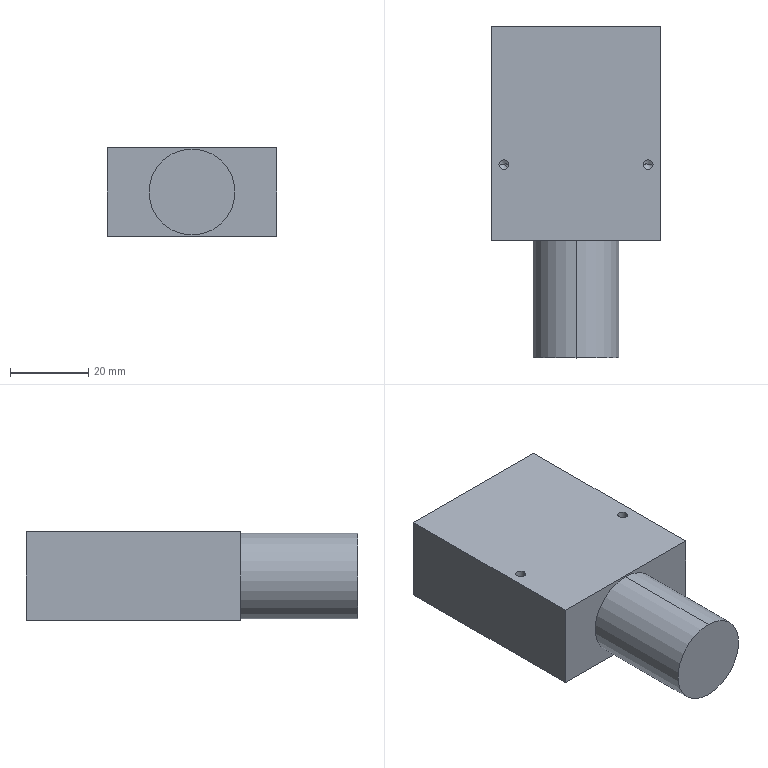Part | STEP file | Guide wheel mechanism revised.sldasm-Part-48 | 1 solid | 17 faces | box 43.5 x 85 x 22.7 mm | volume 65638 mm3 | plane 7 | cylinder 6 | cone 4 | commonest cylinder face diameters 2.5 x4 22 x2
STEP:
#1=CARTESIAN_POINT('',(0.,-30.,-11.));
#2=VERTEX_POINT('',#1);
#3=CARTESIAN_POINT('',(0.,-30.,11.));
#4=VERTEX_POINT('',#3);
#5=CARTESIAN_POINT('',(0.,-30.,0.));
#6=DIRECTION('',(0.,-1.,0.));
#7=DIRECTION('',(0.,0.,-1.));
#8=AXIS2_PLACEMENT_3D('',#5,#6,#7);
#9=CIRCLE('',#8,11.);
#10=EDGE_CURVE('',#2,#4,#9,.T.);
#11=ORIENTED_EDGE('',*,*,#10,.F.);
#12=CARTESIAN_POINT('',(0.,0.,-11.));
#13=VERTEX_POINT('',#12);
#14=CARTESIAN_POINT('',(0.,-30.,-11.));
#15=DIRECTION('',(0.,1.,0.));
#16=VECTOR('',#15,1000.);
#17=LINE('',#14,#16);
#18=EDGE_CURVE('',#2,#13,#17,.T.);
#19=ORIENTED_EDGE('',*,*,#18,.T.);
#20=CARTESIAN_POINT('',(0.,0.,11.));
#21=VERTEX_POINT('',#20);
#22=CARTESIAN_POINT('',(0.,0.,0.));
#23=DIRECTION('',(0.,-1.,0.));
#24=DIRECTION('',(0.,0.,-1.));
#25=AXIS2_PLACEMENT_3D('',#22,#23,#24);
#26=CIRCLE('',#25,11.);
#27=EDGE_CURVE('',#13,#21,#26,.T.);
#28=ORIENTED_EDGE('',*,*,#27,.T.);
#29=CARTESIAN_POINT('',(0.,-30.,11.));
#30=DIRECTION('',(0.,1.,0.));
#31=VECTOR('',#30,1000.);
#32=LINE('',#29,#31);
#33=EDGE_CURVE('',#4,#21,#32,.T.);
#34=ORIENTED_EDGE('',*,*,#33,.F.);
#35=EDGE_LOOP('',(#11,#19,#28,#34));
#36=FACE_OUTER_BOUND('',#35,.T.);
#37=CARTESIAN_POINT('',(0.,-30.,0.));
#38=DIRECTION('',(0.,1.,0.));
#39=DIRECTION('',(0.,0.,1.));
#40=AXIS2_PLACEMENT_3D('',#37,#38,#39);
#41=CYLINDRICAL_SURFACE('',#40,11.);
#42=ADVANCED_FACE('',(#36),#41,.T.);
#43=CARTESIAN_POINT('',(-19.75,19.5,3.85));
#44=VERTEX_POINT('',#43);
#45=CARTESIAN_POINT('',(-17.25,19.5,3.85));
#46=VERTEX_POINT('',#45);
#47=CARTESIAN_POINT('',(-18.5,19.5,3.85));
#48=DIRECTION('',(0.,0.,1.));
#49=DIRECTION('',(1.,0.,0.));
#50=AXIS2_PLACEMENT_3D('',#47,#48,#49);
#51=CIRCLE('',#50,1.25);
#52=EDGE_CURVE('',#44,#46,#51,.T.);
#53=ORIENTED_EDGE('',*,*,#52,.F.);
#54=CARTESIAN_POINT('',(-19.75,19.5,11.35));
#55=VERTEX_POINT('',#54);
#56=CARTESIAN_POINT('',(-19.75,19.5,11.35));
#57=DIRECTION('',(0.,0.,1.));
#58=VECTOR('',#57,1000.);
#59=LINE('',#56,#58);
#60=EDGE_CURVE('',#44,#55,#59,.T.);
#61=ORIENTED_EDGE('',*,*,#60,.T.);
#62=CARTESIAN_POINT('',(-17.25,19.5,11.35));
#63=VERTEX_POINT('',#62);
#64=CARTESIAN_POINT('',(-18.5,19.5,11.35));
#65=DIRECTION('',(0.,0.,1.));
#66=DIRECTION('',(1.,0.,0.));
#67=AXIS2_PLACEMENT_3D('',#64,#65,#66);
#68=CIRCLE('',#67,1.25);
#69=EDGE_CURVE('',#55,#63,#68,.T.);
#70=ORIENTED_EDGE('',*,*,#69,.T.);
#71=CARTESIAN_POINT('',(-17.25,19.5,11.35));
#72=DIRECTION('',(0.,0.,1.));
#73=VECTOR('',#72,1000.);
#74=LINE('',#71,#73);
#75=EDGE_CURVE('',#46,#63,#74,.T.);
#76=ORIENTED_EDGE('',*,*,#75,.F.);
#77=EDGE_LOOP('',(#53,#61,#70,#76));
#78=FACE_OUTER_BOUND('',#77,.T.);
#79=CARTESIAN_POINT('',(-18.5,19.5,11.35));
#80=DIRECTION('',(0.,0.,1.));
#81=DIRECTION('',(1.,0.,0.));
#82=AXIS2_PLACEMENT_3D('',#79,#80,#81);
#83=CYLINDRICAL_SURFACE('',#82,1.25);
#84=ADVANCED_FACE('',(#78),#83,.F.);
#85=CARTESIAN_POINT('',(-18.5,19.5,3.099));
#86=VERTEX_POINT('',#85);
#87=CARTESIAN_POINT('',(-17.25,19.5,3.85));
#88=DIRECTION('',(0.8572,0.,0.515));
#89=VECTOR('',#88,1000.);
#90=LINE('',#87,#89);
#91=EDGE_CURVE('',#86,#46,#90,.T.);
#92=ORIENTED_EDGE('',*,*,#91,.F.);
#93=CARTESIAN_POINT('',(-19.75,19.5,3.85));
#94=DIRECTION('',(-0.8572,0.,0.515));
#95=VECTOR('',#94,1000.);
#96=LINE('',#93,#95);
#97=EDGE_CURVE('',#86,#44,#96,.T.);
#98=ORIENTED_EDGE('',*,*,#97,.T.);
#99=ORIENTED_EDGE('',*,*,#52,.T.);
#100=EDGE_LOOP('',(#92,#98,#99));
#101=FACE_OUTER_BOUND('',#100,.T.);
#102=CARTESIAN_POINT('',(-18.5,19.5,3.85));
#103=DIRECTION('',(0.,0.,1.));
#104=DIRECTION('',(1.,0.,0.));
#105=AXIS2_PLACEMENT_3D('',#102,#103,#104);
#106=CONICAL_SURFACE('',#105,1.25,1.03);
#107=ADVANCED_FACE('',(#101),#106,.F.);
#108=CARTESIAN_POINT('',(17.25,19.5,3.85));
#109=VERTEX_POINT('',#108);
#110=CARTESIAN_POINT('',(19.75,19.5,3.85));
#111=VERTEX_POINT('',#110);
#112=CARTESIAN_POINT('',(18.5,19.5,3.85));
#113=DIRECTION('',(0.,0.,1.));
#114=DIRECTION('',(1.,0.,0.));
#115=AXIS2_PLACEMENT_3D('',#112,#113,#114);
#116=CIRCLE('',#115,1.25);
#117=EDGE_CURVE('',#109,#111,#116,.T.);
#118=ORIENTED_EDGE('',*,*,#117,.F.);
#119=CARTESIAN_POINT('',(17.25,19.5,11.35));
#120=VERTEX_POINT('',#119);
#121=CARTESIAN_POINT('',(17.25,19.5,11.35));
#122=DIRECTION('',(0.,0.,1.));
#123=VECTOR('',#122,1000.);
#124=LINE('',#121,#123);
#125=EDGE_CURVE('',#109,#120,#124,.T.);
#126=ORIENTED_EDGE('',*,*,#125,.T.);
#127=CARTESIAN_POINT('',(19.75,19.5,11.35));
#128=VERTEX_POINT('',#127);
#129=CARTESIAN_POINT('',(18.5,19.5,11.35));
#130=DIRECTION('',(0.,0.,1.));
#131=DIRECTION('',(1.,0.,0.));
#132=AXIS2_PLACEMENT_3D('',#129,#130,#131);
#133=CIRCLE('',#132,1.25);
#134=EDGE_CURVE('',#120,#128,#133,.T.);
#135=ORIENTED_EDGE('',*,*,#134,.T.);
#136=CARTESIAN_POINT('',(19.75,19.5,11.35));
#137=DIRECTION('',(0.,0.,1.));
#138=VECTOR('',#137,1000.);
#139=LINE('',#136,#138);
#140=EDGE_CURVE('',#111,#128,#139,.T.);
#141=ORIENTED_EDGE('',*,*,#140,.F.);
#142=EDGE_LOOP('',(#118,#126,#135,#141));
#143=FACE_OUTER_BOUND('',#142,.T.);
#144=CARTESIAN_POINT('',(18.5,19.5,11.35));
#145=DIRECTION('',(0.,0.,1.));
#146=DIRECTION('',(1.,0.,0.));
#147=AXIS2_PLACEMENT_3D('',#144,#145,#146);
#148=CYLINDRICAL_SURFACE('',#147,1.25);
#149=ADVANCED_FACE('',(#143),#148,.F.);
#150=CARTESIAN_POINT('',(18.5,19.5,3.099));
#151=VERTEX_POINT('',#150);
#152=CARTESIAN_POINT('',(19.75,19.5,3.85));
#153=DIRECTION('',(0.8572,0.,0.515));
#154=VECTOR('',#153,1000.);
#155=LINE('',#152,#154);
#156=EDGE_CURVE('',#151,#111,#155,.T.);
#157=ORIENTED_EDGE('',*,*,#156,.F.);
#158=CARTESIAN_POINT('',(17.25,19.5,3.85));
#159=DIRECTION('',(-0.8572,0.,0.515));
#160=VECTOR('',#159,1000.);
#161=LINE('',#158,#160);
#162=EDGE_CURVE('',#151,#109,#161,.T.);
#163=ORIENTED_EDGE('',*,*,#162,.T.);
#164=ORIENTED_EDGE('',*,*,#117,.T.);
#165=EDGE_LOOP('',(#157,#163,#164));
#166=FACE_OUTER_BOUND('',#165,.T.);
#167=CARTESIAN_POINT('',(18.5,19.5,3.85));
#168=DIRECTION('',(0.,0.,1.));
#169=DIRECTION('',(1.,0.,0.));
#170=AXIS2_PLACEMENT_3D('',#167,#168,#169);
#171=CONICAL_SURFACE('',#170,1.25,1.03);
#172=ADVANCED_FACE('',(#166),#171,.F.);
#173=CARTESIAN_POINT('',(21.75,0.,11.35));
#174=VERTEX_POINT('',#173);
#175=CARTESIAN_POINT('',(21.75,0.,-11.35));
#176=VERTEX_POINT('',#175);
#177=CARTESIAN_POINT('',(21.75,0.,11.35));
#178=DIRECTION('',(0.,0.,-1.));
#179=VECTOR('',#178,1000.);
#180=LINE('',#177,#179);
#181=EDGE_CURVE('',#174,#176,#180,.T.);
#182=ORIENTED_EDGE('',*,*,#181,.F.);
#183=CARTESIAN_POINT('',(-21.75,0.,11.35));
#184=VERTEX_POINT('',#183);
#185=CARTESIAN_POINT('',(-21.75,0.,11.35));
#186=DIRECTION('',(1.,0.,0.));
#187=VECTOR('',#186,1000.);
#188=LINE('',#185,#187);
#189=EDGE_CURVE('',#184,#174,#188,.T.);
#190=ORIENTED_EDGE('',*,*,#189,.F.);
#191=CARTESIAN_POINT('',(-21.75,0.,-11.35));
#192=VERTEX_POINT('',#191);
#193=CARTESIAN_POINT('',(-21.75,0.,11.35));
#194=DIRECTION('',(0.,0.,1.));
#195=VECTOR('',#194,1000.);
#196=LINE('',#193,#195);
#197=EDGE_CURVE('',#192,#184,#196,.T.);
#198=ORIENTED_EDGE('',*,*,#197,.F.);
#199=CARTESIAN_POINT('',(-21.75,0.,-11.35));
#200=DIRECTION('',(-1.,0.,0.));
#201=VECTOR('',#200,1000.);
#202=LINE('',#199,#201);
#203=EDGE_CURVE('',#176,#192,#202,.T.);
#204=ORIENTED_EDGE('',*,*,#203,.F.);
#205=EDGE_LOOP('',(#182,#190,#198,#204));
#206=FACE_OUTER_BOUND('',#205,.T.);
#207=CARTESIAN_POINT('',(0.,0.,0.));
#208=DIRECTION('',(0.,-1.,0.));
#209=DIRECTION('',(0.,0.,-1.));
#210=AXIS2_PLACEMENT_3D('',#207,#208,#209);
#211=CIRCLE('',#210,11.);
#212=EDGE_CURVE('',#21,#13,#211,.T.);
#213=ORIENTED_EDGE('',*,*,#212,.F.);
#214=ORIENTED_EDGE('',*,*,#27,.F.);
#215=EDGE_LOOP('',(#213,#214));
#216=FACE_BOUND('',#215,.T.);
#217=CARTESIAN_POINT('',(0.,0.,0.));
#218=DIRECTION('',(0.,-1.,0.));
#219=DIRECTION('',(0.,0.,-1.));
#220=AXIS2_PLACEMENT_3D('',#217,#218,#219);
#221=PLANE('',#220);
#222=ADVANCED_FACE('',(#206,#216),#221,.T.);
#223=ORIENTED_EDGE('',*,*,#181,.T.);
#224=CARTESIAN_POINT('',(21.75,55.,-11.35));
#225=VERTEX_POINT('',#224);
#226=CARTESIAN_POINT('',(21.75,55.,-11.35));
#227=DIRECTION('',(0.,-1.,0.));
#228=VECTOR('',#227,1000.);
#229=LINE('',#226,#228);
#230=EDGE_CURVE('',#225,#176,#229,.T.);
#231=ORIENTED_EDGE('',*,*,#230,.F.);
#232=CARTESIAN_POINT('',(21.75,55.,11.35));
#233=VERTEX_POINT('',#232);
#234=CARTESIAN_POINT('',(21.75,55.,11.35));
#235=DIRECTION('',(0.,0.,-1.));
#236=VECTOR('',#235,1000.);
#237=LINE('',#234,#236);
#238=EDGE_CURVE('',#233,#225,#237,.T.);
#239=ORIENTED_EDGE('',*,*,#238,.F.);
#240=CARTESIAN_POINT('',(21.75,55.,11.35));
#241=DIRECTION('',(0.,-1.,0.));
#242=VECTOR('',#241,1000.);
#243=LINE('',#240,#242);
#244=EDGE_CURVE('',#233,#174,#243,.T.);
#245=ORIENTED_EDGE('',*,*,#244,.T.);
#246=EDGE_LOOP('',(#223,#231,#239,#245));
#247=FACE_OUTER_BOUND('',#246,.T.);
#248=CARTESIAN_POINT('',(21.75,55.,11.35));
#249=DIRECTION('',(-1.,0.,0.));
#250=DIRECTION('',(0.,0.,1.));
#251=AXIS2_PLACEMENT_3D('',#248,#249,#250);
#252=PLANE('',#251);
#253=ADVANCED_FACE('',(#247),#252,.F.);
#254=ORIENTED_EDGE('',*,*,#203,.T.);
#255=CARTESIAN_POINT('',(-21.75,55.,-11.35));
#256=VERTEX_POINT('',#255);
#257=CARTESIAN_POINT('',(-21.75,55.,-11.35));
#258=DIRECTION('',(0.,-1.,0.));
#259=VECTOR('',#258,1000.);
#260=LINE('',#257,#259);
#261=EDGE_CURVE('',#256,#192,#260,.T.);
#262=ORIENTED_EDGE('',*,*,#261,.F.);
#263=CARTESIAN_POINT('',(-21.75,55.,-11.35));
#264=DIRECTION('',(-1.,0.,0.));
#265=VECTOR('',#264,1000.);
#266=LINE('',#263,#265);
#267=EDGE_CURVE('',#225,#256,#266,.T.);
#268=ORIENTED_EDGE('',*,*,#267,.F.);
#269=ORIENTED_EDGE('',*,*,#230,.T.);
#270=EDGE_LOOP('',(#254,#262,#268,#269));
#271=FACE_OUTER_BOUND('',#270,.T.);
#272=CARTESIAN_POINT('',(-21.75,55.,-11.35));
#273=DIRECTION('',(0.,0.,1.));
#274=DIRECTION('',(1.,0.,0.));
#275=AXIS2_PLACEMENT_3D('',#272,#273,#274);
#276=PLANE('',#275);
#277=ADVANCED_FACE('',(#271),#276,.F.);
#278=ORIENTED_EDGE('',*,*,#197,.T.);
#279=CARTESIAN_POINT('',(-21.75,55.,11.35));
#280=VERTEX_POINT('',#279);
#281=CARTESIAN_POINT('',(-21.75,55.,11.35));
#282=DIRECTION('',(0.,-1.,0.));
#283=VECTOR('',#282,1000.);
#284=LINE('',#281,#283);
#285=EDGE_CURVE('',#280,#184,#284,.T.);
#286=ORIENTED_EDGE('',*,*,#285,.F.);
#287=CARTESIAN_POINT('',(-21.75,55.,11.35));
#288=DIRECTION('',(0.,0.,1.));
#289=VECTOR('',#288,1000.);
#290=LINE('',#287,#289);
#291=EDGE_CURVE('',#256,#280,#290,.T.);
#292=ORIENTED_EDGE('',*,*,#291,.F.);
#293=ORIENTED_EDGE('',*,*,#261,.T.);
#294=EDGE_LOOP('',(#278,#286,#292,#293));
#295=FACE_OUTER_BOUND('',#294,.T.);
#296=CARTESIAN_POINT('',(-21.75,55.,11.35));
#297=DIRECTION('',(1.,0.,0.));
#298=DIRECTION('',(0.,0.,-1.));
#299=AXIS2_PLACEMENT_3D('',#296,#297,#298);
#300=PLANE('',#299);
#301=ADVANCED_FACE('',(#295),#300,.F.);
#302=CARTESIAN_POINT('',(-18.5,19.5,11.35));
#303=DIRECTION('',(0.,0.,1.));
#304=DIRECTION('',(1.,0.,0.));
#305=AXIS2_PLACEMENT_3D('',#302,#303,#304);
#306=CIRCLE('',#305,1.25);
#307=EDGE_CURVE('',#63,#55,#306,.T.);
#308=ORIENTED_EDGE('',*,*,#307,.F.);
#309=ORIENTED_EDGE('',*,*,#69,.F.);
#310=EDGE_LOOP('',(#308,#309));
#311=FACE_BOUND('',#310,.T.);
#312=CARTESIAN_POINT('',(18.5,19.5,11.35));
#313=DIRECTION('',(0.,0.,1.));
#314=DIRECTION('',(1.,0.,0.));
#315=AXIS2_PLACEMENT_3D('',#312,#313,#314);
#316=CIRCLE('',#315,1.25);
#317=EDGE_CURVE('',#128,#120,#316,.T.);
#318=ORIENTED_EDGE('',*,*,#317,.F.);
#319=ORIENTED_EDGE('',*,*,#134,.F.);
#320=EDGE_LOOP('',(#318,#319));
#321=FACE_BOUND('',#320,.T.);
#322=ORIENTED_EDGE('',*,*,#189,.T.);
#323=ORIENTED_EDGE('',*,*,#244,.F.);
#324=CARTESIAN_POINT('',(-21.75,55.,11.35));
#325=DIRECTION('',(1.,0.,0.));
#326=VECTOR('',#325,1000.);
#327=LINE('',#324,#326);
#328=EDGE_CURVE('',#280,#233,#327,.T.);
#329=ORIENTED_EDGE('',*,*,#328,.F.);
#330=ORIENTED_EDGE('',*,*,#285,.T.);
#331=EDGE_LOOP('',(#322,#323,#329,#330));
#332=FACE_OUTER_BOUND('',#331,.T.);
#333=CARTESIAN_POINT('',(-21.75,55.,11.35));
#334=DIRECTION('',(0.,0.,-1.));
#335=DIRECTION('',(-1.,0.,0.));
#336=AXIS2_PLACEMENT_3D('',#333,#334,#335);
#337=PLANE('',#336);
#338=ADVANCED_FACE('',(#311,#321,#332),#337,.F.);
#339=ORIENTED_EDGE('',*,*,#238,.T.);
#340=ORIENTED_EDGE('',*,*,#267,.T.);
#341=ORIENTED_EDGE('',*,*,#291,.T.);
#342=ORIENTED_EDGE('',*,*,#328,.T.);
#343=EDGE_LOOP('',(#339,#340,#341,#342));
#344=FACE_OUTER_BOUND('',#343,.T.);
#345=CARTESIAN_POINT('',(0.,55.,0.));
#346=DIRECTION('',(0.,-1.,0.));
#347=DIRECTION('',(0.,0.,-1.));
#348=AXIS2_PLACEMENT_3D('',#345,#346,#347);
#349=PLANE('',#348);
#350=ADVANCED_FACE('',(#344),#349,.F.);
#351=ORIENTED_EDGE('',*,*,#162,.F.);
#352=ORIENTED_EDGE('',*,*,#156,.T.);
#353=CARTESIAN_POINT('',(18.5,19.5,3.85));
#354=DIRECTION('',(0.,0.,1.));
#355=DIRECTION('',(1.,0.,0.));
#356=AXIS2_PLACEMENT_3D('',#353,#354,#355);
#357=CIRCLE('',#356,1.25);
#358=EDGE_CURVE('',#111,#109,#357,.T.);
#359=ORIENTED_EDGE('',*,*,#358,.T.);
#360=EDGE_LOOP('',(#351,#352,#359));
#361=FACE_OUTER_BOUND('',#360,.T.);
#362=CARTESIAN_POINT('',(18.5,19.5,3.85));
#363=DIRECTION('',(0.,0.,1.));
#364=DIRECTION('',(1.,0.,0.));
#365=AXIS2_PLACEMENT_3D('',#362,#363,#364);
#366=CONICAL_SURFACE('',#365,1.25,1.03);
#367=ADVANCED_FACE('',(#361),#366,.F.);
#368=ORIENTED_EDGE('',*,*,#125,.F.);
#369=ORIENTED_EDGE('',*,*,#358,.F.);
#370=ORIENTED_EDGE('',*,*,#140,.T.);
#371=ORIENTED_EDGE('',*,*,#317,.T.);
#372=EDGE_LOOP('',(#368,#369,#370,#371));
#373=FACE_OUTER_BOUND('',#372,.T.);
#374=CARTESIAN_POINT('',(18.5,19.5,11.35));
#375=DIRECTION('',(0.,0.,1.));
#376=DIRECTION('',(1.,0.,0.));
#377=AXIS2_PLACEMENT_3D('',#374,#375,#376);
#378=CYLINDRICAL_SURFACE('',#377,1.25);
#379=ADVANCED_FACE('',(#373),#378,.F.);
#380=ORIENTED_EDGE('',*,*,#97,.F.);
#381=ORIENTED_EDGE('',*,*,#91,.T.);
#382=CARTESIAN_POINT('',(-18.5,19.5,3.85));
#383=DIRECTION('',(0.,0.,1.));
#384=DIRECTION('',(1.,0.,0.));
#385=AXIS2_PLACEMENT_3D('',#382,#383,#384);
#386=CIRCLE('',#385,1.25);
#387=EDGE_CURVE('',#46,#44,#386,.T.);
#388=ORIENTED_EDGE('',*,*,#387,.T.);
#389=EDGE_LOOP('',(#380,#381,#388));
#390=FACE_OUTER_BOUND('',#389,.T.);
#391=CARTESIAN_POINT('',(-18.5,19.5,3.85));
#392=DIRECTION('',(0.,0.,1.));
#393=DIRECTION('',(1.,0.,0.));
#394=AXIS2_PLACEMENT_3D('',#391,#392,#393);
#395=CONICAL_SURFACE('',#394,1.25,1.03);
#396=ADVANCED_FACE('',(#390),#395,.F.);
#397=ORIENTED_EDGE('',*,*,#60,.F.);
#398=ORIENTED_EDGE('',*,*,#387,.F.);
#399=ORIENTED_EDGE('',*,*,#75,.T.);
#400=ORIENTED_EDGE('',*,*,#307,.T.);
#401=EDGE_LOOP('',(#397,#398,#399,#400));
#402=FACE_OUTER_BOUND('',#401,.T.);
#403=CARTESIAN_POINT('',(-18.5,19.5,11.35));
#404=DIRECTION('',(0.,0.,1.));
#405=DIRECTION('',(1.,0.,0.));
#406=AXIS2_PLACEMENT_3D('',#403,#404,#405);
#407=CYLINDRICAL_SURFACE('',#406,1.25);
#408=ADVANCED_FACE('',(#402),#407,.F.);
#409=ORIENTED_EDGE('',*,*,#18,.F.);
#410=CARTESIAN_POINT('',(0.,-30.,0.));
#411=DIRECTION('',(0.,-1.,0.));
#412=DIRECTION('',(0.,0.,-1.));
#413=AXIS2_PLACEMENT_3D('',#410,#411,#412);
#414=CIRCLE('',#413,11.);
#415=EDGE_CURVE('',#4,#2,#414,.T.);
#416=ORIENTED_EDGE('',*,*,#415,.F.);
#417=ORIENTED_EDGE('',*,*,#33,.T.);
#418=ORIENTED_EDGE('',*,*,#212,.T.);
#419=EDGE_LOOP('',(#409,#416,#417,#418));
#420=FACE_OUTER_BOUND('',#419,.T.);
#421=CARTESIAN_POINT('',(0.,-30.,0.));
#422=DIRECTION('',(0.,1.,0.));
#423=DIRECTION('',(0.,0.,1.));
#424=AXIS2_PLACEMENT_3D('',#421,#422,#423);
#425=CYLINDRICAL_SURFACE('',#424,11.);
#426=ADVANCED_FACE('',(#420),#425,.T.);
#427=ORIENTED_EDGE('',*,*,#415,.T.);
#428=ORIENTED_EDGE('',*,*,#10,.T.);
#429=EDGE_LOOP('',(#427,#428));
#430=FACE_OUTER_BOUND('',#429,.T.);
#431=CARTESIAN_POINT('',(0.,-30.,0.));
#432=DIRECTION('',(0.,-1.,0.));
#433=DIRECTION('',(0.,0.,-1.));
#434=AXIS2_PLACEMENT_3D('',#431,#432,#433);
#435=PLANE('',#434);
#436=ADVANCED_FACE('',(#430),#435,.T.);
#437=CLOSED_SHELL('',(#42,#84,#107,#149,#172,#222,#253,#277,#301,#338,#350,#367,#379,#396,#408,#426,#436));
#438=MANIFOLD_SOLID_BREP('',#437);
#439=CARTESIAN_POINT('',(0.,0.,0.));
#440=DIRECTION('',(0.,0.,1.));
#441=DIRECTION('',(1.,0.,0.));
#442=AXIS2_PLACEMENT_3D('',#439,#440,#441);
#443=(LENGTH_UNIT()NAMED_UNIT(*)SI_UNIT(.MILLI.,.METRE.));
#444=UNCERTAINTY_MEASURE_WITH_UNIT(LENGTH_MEASURE(0.00001),#443,'','');
#445=(NAMED_UNIT(*)PLANE_ANGLE_UNIT()SI_UNIT($,.RADIAN.));
#446=(NAMED_UNIT(*)SI_UNIT($,.STERADIAN.)SOLID_ANGLE_UNIT());
#447=(GEOMETRIC_REPRESENTATION_CONTEXT(3)GLOBAL_UNCERTAINTY_ASSIGNED_CONTEXT((#444))GLOBAL_UNIT_ASSIGNED_CONTEXT((#443,#445,#446))REPRESENTATION_CONTEXT('',''));
#448=ADVANCED_BREP_SHAPE_REPRESENTATION('',(#438,#442),#447);